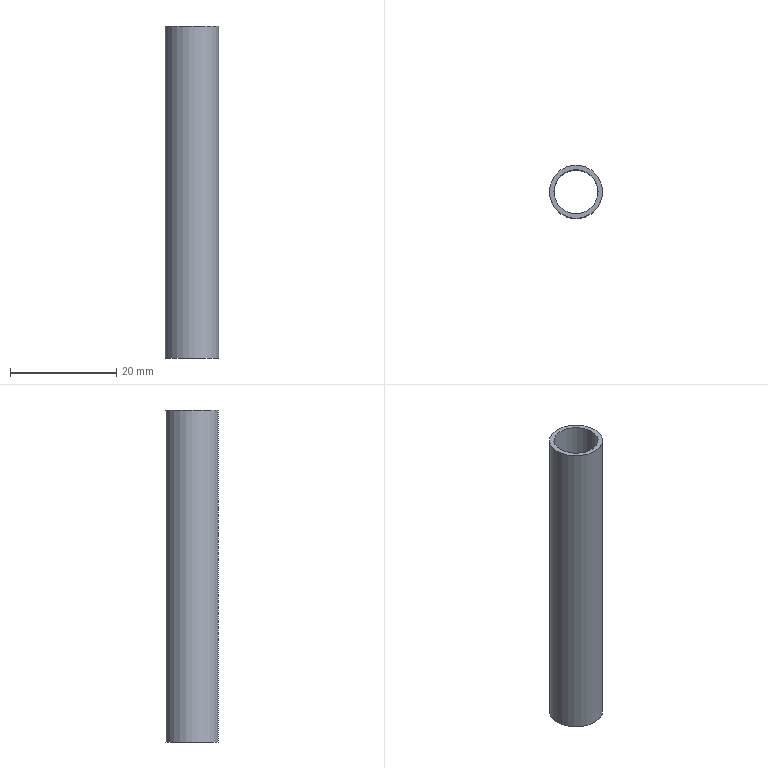Part | NX | 1 solid | 4 faces | box 10 x 10 x 62.5 mm | volume 1527 mm3 | cylinder 2 | plane 2 | commonest cylinder face diameters 8.3 x1 10 x1
STEP:
#1=CARTESIAN_POINT('',(5.,0.,0.));
#2=VERTEX_POINT('',#1);
#3=CARTESIAN_POINT('',(0.,0.,0.));
#4=DIRECTION('',(0.,0.,1.));
#5=DIRECTION('',(1.,0.,0.));
#6=AXIS2_PLACEMENT_3D('',#3,#4,#5);
#7=CIRCLE('',#6,5.);
#8=EDGE_CURVE('',#2,#2,#7,.T.);
#9=ORIENTED_EDGE('',*,*,#8,.T.);
#10=EDGE_LOOP('',(#9));
#11=FACE_BOUND('',#10,.T.);
#12=CARTESIAN_POINT('',(5.,0.,62.5));
#13=VERTEX_POINT('',#12);
#14=CARTESIAN_POINT('',(0.,0.,62.5));
#15=DIRECTION('',(0.,0.,1.));
#16=DIRECTION('',(1.,0.,0.));
#17=AXIS2_PLACEMENT_3D('',#14,#15,#16);
#18=CIRCLE('',#17,5.);
#19=EDGE_CURVE('',#13,#13,#18,.F.);
#20=ORIENTED_EDGE('',*,*,#19,.T.);
#21=EDGE_LOOP('',(#20));
#22=FACE_BOUND('',#21,.T.);
#23=CARTESIAN_POINT('',(0.,0.,0.));
#24=DIRECTION('',(0.,0.,1.));
#25=DIRECTION('',(1.,0.,0.));
#26=AXIS2_PLACEMENT_3D('',#23,#24,#25);
#27=CYLINDRICAL_SURFACE('',#26,5.);
#28=ADVANCED_FACE('',(#11,#22),#27,.T.);
#29=CARTESIAN_POINT('',(4.15,0.,0.));
#30=VERTEX_POINT('',#29);
#31=CARTESIAN_POINT('',(0.,0.,0.));
#32=DIRECTION('',(0.,0.,1.));
#33=DIRECTION('',(1.,0.,0.));
#34=AXIS2_PLACEMENT_3D('',#31,#32,#33);
#35=CIRCLE('',#34,4.15);
#36=EDGE_CURVE('',#30,#30,#35,.T.);
#37=ORIENTED_EDGE('',*,*,#36,.T.);
#38=EDGE_LOOP('',(#37));
#39=FACE_BOUND('',#38,.T.);
#40=ORIENTED_EDGE('',*,*,#8,.F.);
#41=EDGE_LOOP('',(#40));
#42=FACE_BOUND('',#41,.T.);
#43=CARTESIAN_POINT('',(0.,0.,0.));
#44=DIRECTION('',(0.,0.,-1.));
#45=DIRECTION('',(-1.,0.,0.));
#46=AXIS2_PLACEMENT_3D('',#43,#44,#45);
#47=PLANE('',#46);
#48=ADVANCED_FACE('',(#39,#42),#47,.T.);
#49=CARTESIAN_POINT('',(4.15,0.,62.5));
#50=VERTEX_POINT('',#49);
#51=CARTESIAN_POINT('',(0.,0.,62.5));
#52=DIRECTION('',(0.,0.,1.));
#53=DIRECTION('',(1.,0.,0.));
#54=AXIS2_PLACEMENT_3D('',#51,#52,#53);
#55=CIRCLE('',#54,4.15);
#56=EDGE_CURVE('',#50,#50,#55,.T.);
#57=ORIENTED_EDGE('',*,*,#56,.F.);
#58=EDGE_LOOP('',(#57));
#59=FACE_BOUND('',#58,.T.);
#60=ORIENTED_EDGE('',*,*,#19,.F.);
#61=EDGE_LOOP('',(#60));
#62=FACE_BOUND('',#61,.T.);
#63=CARTESIAN_POINT('',(0.,0.,62.5));
#64=DIRECTION('',(0.,0.,-1.));
#65=DIRECTION('',(-1.,0.,0.));
#66=AXIS2_PLACEMENT_3D('',#63,#64,#65);
#67=PLANE('',#66);
#68=ADVANCED_FACE('',(#59,#62),#67,.F.);
#69=ORIENTED_EDGE('',*,*,#36,.F.);
#70=EDGE_LOOP('',(#69));
#71=FACE_BOUND('',#70,.T.);
#72=ORIENTED_EDGE('',*,*,#56,.T.);
#73=EDGE_LOOP('',(#72));
#74=FACE_BOUND('',#73,.T.);
#75=CARTESIAN_POINT('',(0.,0.,0.));
#76=DIRECTION('',(0.,0.,1.));
#77=DIRECTION('',(1.,0.,0.));
#78=AXIS2_PLACEMENT_3D('',#75,#76,#77);
#79=CYLINDRICAL_SURFACE('',#78,4.15);
#80=ADVANCED_FACE('',(#71,#74),#79,.F.);
#81=CLOSED_SHELL('',(#28,#48,#68,#80));
#82=MANIFOLD_SOLID_BREP('',#81);
#83=(LENGTH_UNIT()NAMED_UNIT(*)SI_UNIT(.MILLI.,.METRE.));
#84=UNCERTAINTY_MEASURE_WITH_UNIT(LENGTH_MEASURE(0.00001),#83,'','');
#85=(NAMED_UNIT(*)PLANE_ANGLE_UNIT()SI_UNIT($,.RADIAN.));
#86=(NAMED_UNIT(*)SI_UNIT($,.STERADIAN.)SOLID_ANGLE_UNIT());
#87=(GEOMETRIC_REPRESENTATION_CONTEXT(3)GLOBAL_UNCERTAINTY_ASSIGNED_CONTEXT((#84))GLOBAL_UNIT_ASSIGNED_CONTEXT((#83,#85,#86))REPRESENTATION_CONTEXT('',''));
#88=ADVANCED_BREP_SHAPE_REPRESENTATION('',(#82),#87);